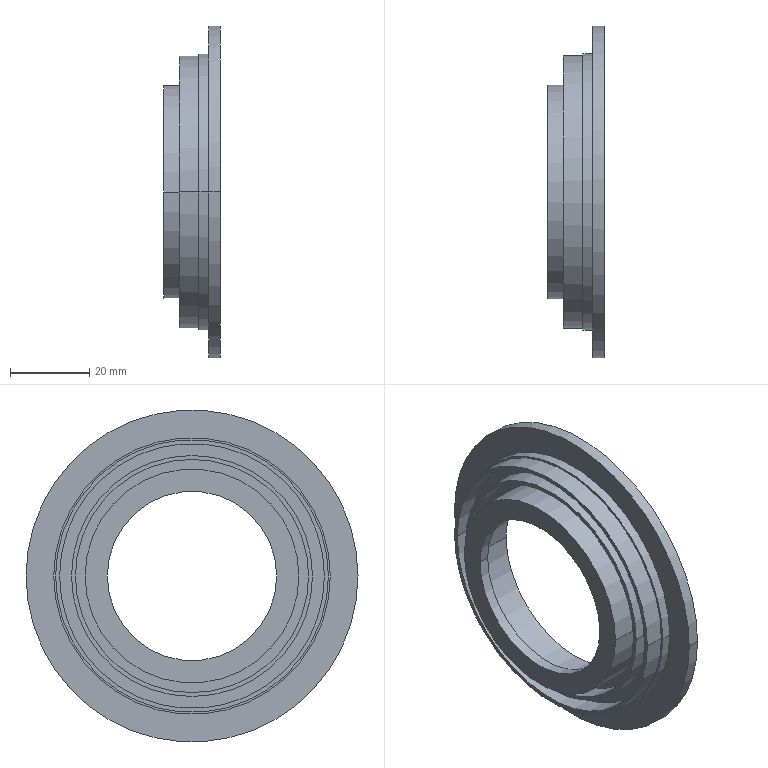Part | SolidWorks | features ICE 1, Revolution 1 | 1 solid | 30 faces | box 14.383 x 84 x 84 mm | volume 20141 mm3 | cylinder 20 | plane 10 | commonest cylinder face diameters 42.865 x2 49.1 x2 54.1 x2 59 x2 61 x2 62.852 x2
STEP:
#1=CARTESIAN_POINT('',(99.508,-34.5,0.));
#2=VERTEX_POINT('',#1);
#3=CARTESIAN_POINT('',(99.508,34.5,0.));
#4=VERTEX_POINT('',#3);
#5=CARTESIAN_POINT('',(99.508,0.,0.));
#6=DIRECTION('',(-1.,0.,0.));
#7=DIRECTION('',(0.,-1.,0.));
#8=AXIS2_PLACEMENT_3D('',#5,#6,#7);
#9=CIRCLE('',#8,34.5);
#10=EDGE_CURVE('',#2,#4,#9,.T.);
#11=ORIENTED_EDGE('',*,*,#10,.F.);
#12=CARTESIAN_POINT('',(104.508,-34.5,0.));
#13=VERTEX_POINT('',#12);
#14=CARTESIAN_POINT('',(99.508,-34.5,0.));
#15=DIRECTION('',(1.,0.,0.));
#16=VECTOR('',#15,1000.);
#17=LINE('',#14,#16);
#18=EDGE_CURVE('',#2,#13,#17,.T.);
#19=ORIENTED_EDGE('',*,*,#18,.T.);
#20=CARTESIAN_POINT('',(104.508,34.5,0.));
#21=VERTEX_POINT('',#20);
#22=CARTESIAN_POINT('',(104.508,0.,0.));
#23=DIRECTION('',(-1.,0.,0.));
#24=DIRECTION('',(0.,-1.,0.));
#25=AXIS2_PLACEMENT_3D('',#22,#23,#24);
#26=CIRCLE('',#25,34.5);
#27=EDGE_CURVE('',#13,#21,#26,.T.);
#28=ORIENTED_EDGE('',*,*,#27,.T.);
#29=CARTESIAN_POINT('',(99.508,34.5,0.));
#30=DIRECTION('',(1.,0.,0.));
#31=VECTOR('',#30,1000.);
#32=LINE('',#29,#31);
#33=EDGE_CURVE('',#4,#21,#32,.T.);
#34=ORIENTED_EDGE('',*,*,#33,.F.);
#35=EDGE_LOOP('',(#11,#19,#28,#34));
#36=FACE_OUTER_BOUND('',#35,.T.);
#37=CARTESIAN_POINT('',(99.508,0.,0.));
#38=DIRECTION('',(1.,0.,0.));
#39=DIRECTION('',(0.,1.,0.));
#40=AXIS2_PLACEMENT_3D('',#37,#38,#39);
#41=CYLINDRICAL_SURFACE('',#40,34.5);
#42=ADVANCED_FACE('',(#36),#41,.T.);
#43=CARTESIAN_POINT('',(99.508,33.5,0.));
#44=VERTEX_POINT('',#43);
#45=CARTESIAN_POINT('',(99.508,-33.5,0.));
#46=VERTEX_POINT('',#45);
#47=CARTESIAN_POINT('',(99.508,0.,0.));
#48=DIRECTION('',(-1.,0.,0.));
#49=DIRECTION('',(0.,-1.,0.));
#50=AXIS2_PLACEMENT_3D('',#47,#48,#49);
#51=CIRCLE('',#50,33.5);
#52=EDGE_CURVE('',#44,#46,#51,.T.);
#53=ORIENTED_EDGE('',*,*,#52,.T.);
#54=CARTESIAN_POINT('',(104.508,-33.5,0.));
#55=VERTEX_POINT('',#54);
#56=CARTESIAN_POINT('',(99.508,-33.5,0.));
#57=DIRECTION('',(1.,0.,0.));
#58=VECTOR('',#57,1000.);
#59=LINE('',#56,#58);
#60=EDGE_CURVE('',#46,#55,#59,.T.);
#61=ORIENTED_EDGE('',*,*,#60,.T.);
#62=CARTESIAN_POINT('',(104.508,33.5,0.));
#63=VERTEX_POINT('',#62);
#64=CARTESIAN_POINT('',(104.508,0.,0.));
#65=DIRECTION('',(1.,0.,0.));
#66=DIRECTION('',(0.,-1.,0.));
#67=AXIS2_PLACEMENT_3D('',#64,#65,#66);
#68=CIRCLE('',#67,33.5);
#69=EDGE_CURVE('',#55,#63,#68,.T.);
#70=ORIENTED_EDGE('',*,*,#69,.T.);
#71=CARTESIAN_POINT('',(99.508,33.5,0.));
#72=DIRECTION('',(1.,0.,0.));
#73=VECTOR('',#72,1000.);
#74=LINE('',#71,#73);
#75=EDGE_CURVE('',#44,#63,#74,.T.);
#76=ORIENTED_EDGE('',*,*,#75,.F.);
#77=EDGE_LOOP('',(#53,#61,#70,#76));
#78=FACE_OUTER_BOUND('',#77,.T.);
#79=CARTESIAN_POINT('',(99.508,0.,0.));
#80=DIRECTION('',(1.,0.,0.));
#81=DIRECTION('',(0.,1.,0.));
#82=AXIS2_PLACEMENT_3D('',#79,#80,#81);
#83=CYLINDRICAL_SURFACE('',#82,33.5);
#84=ADVANCED_FACE('',(#78),#83,.F.);
#85=CARTESIAN_POINT('',(99.508,-30.5,0.));
#86=VERTEX_POINT('',#85);
#87=CARTESIAN_POINT('',(99.508,30.5,0.));
#88=VERTEX_POINT('',#87);
#89=CARTESIAN_POINT('',(99.508,0.,0.));
#90=DIRECTION('',(-1.,0.,0.));
#91=DIRECTION('',(0.,-1.,0.));
#92=AXIS2_PLACEMENT_3D('',#89,#90,#91);
#93=CIRCLE('',#92,30.5);
#94=EDGE_CURVE('',#86,#88,#93,.T.);
#95=ORIENTED_EDGE('',*,*,#94,.F.);
#96=CARTESIAN_POINT('',(104.508,-30.5,0.));
#97=VERTEX_POINT('',#96);
#98=CARTESIAN_POINT('',(99.508,-30.5,0.));
#99=DIRECTION('',(1.,0.,0.));
#100=VECTOR('',#99,1000.);
#101=LINE('',#98,#100);
#102=EDGE_CURVE('',#86,#97,#101,.T.);
#103=ORIENTED_EDGE('',*,*,#102,.T.);
#104=CARTESIAN_POINT('',(104.508,30.5,0.));
#105=VERTEX_POINT('',#104);
#106=CARTESIAN_POINT('',(104.508,0.,0.));
#107=DIRECTION('',(-1.,0.,0.));
#108=DIRECTION('',(0.,-1.,0.));
#109=AXIS2_PLACEMENT_3D('',#106,#107,#108);
#110=CIRCLE('',#109,30.5);
#111=EDGE_CURVE('',#97,#105,#110,.T.);
#112=ORIENTED_EDGE('',*,*,#111,.T.);
#113=CARTESIAN_POINT('',(99.508,30.5,0.));
#114=DIRECTION('',(1.,0.,0.));
#115=VECTOR('',#114,1000.);
#116=LINE('',#113,#115);
#117=EDGE_CURVE('',#88,#105,#116,.T.);
#118=ORIENTED_EDGE('',*,*,#117,.F.);
#119=EDGE_LOOP('',(#95,#103,#112,#118));
#120=FACE_OUTER_BOUND('',#119,.T.);
#121=CARTESIAN_POINT('',(99.508,0.,0.));
#122=DIRECTION('',(1.,0.,0.));
#123=DIRECTION('',(0.,1.,0.));
#124=AXIS2_PLACEMENT_3D('',#121,#122,#123);
#125=CYLINDRICAL_SURFACE('',#124,30.5);
#126=ADVANCED_FACE('',(#120),#125,.T.);
#127=CARTESIAN_POINT('',(99.508,29.5,0.));
#128=VERTEX_POINT('',#127);
#129=CARTESIAN_POINT('',(99.508,-29.5,0.));
#130=VERTEX_POINT('',#129);
#131=CARTESIAN_POINT('',(99.508,0.,0.));
#132=DIRECTION('',(-1.,0.,0.));
#133=DIRECTION('',(0.,-1.,0.));
#134=AXIS2_PLACEMENT_3D('',#131,#132,#133);
#135=CIRCLE('',#134,29.5);
#136=EDGE_CURVE('',#128,#130,#135,.T.);
#137=ORIENTED_EDGE('',*,*,#136,.T.);
#138=CARTESIAN_POINT('',(104.508,-29.5,0.));
#139=VERTEX_POINT('',#138);
#140=CARTESIAN_POINT('',(99.508,-29.5,0.));
#141=DIRECTION('',(1.,0.,0.));
#142=VECTOR('',#141,1000.);
#143=LINE('',#140,#142);
#144=EDGE_CURVE('',#130,#139,#143,.T.);
#145=ORIENTED_EDGE('',*,*,#144,.T.);
#146=CARTESIAN_POINT('',(104.508,29.5,0.));
#147=VERTEX_POINT('',#146);
#148=CARTESIAN_POINT('',(104.508,0.,0.));
#149=DIRECTION('',(1.,0.,0.));
#150=DIRECTION('',(0.,-1.,0.));
#151=AXIS2_PLACEMENT_3D('',#148,#149,#150);
#152=CIRCLE('',#151,29.5);
#153=EDGE_CURVE('',#139,#147,#152,.T.);
#154=ORIENTED_EDGE('',*,*,#153,.T.);
#155=CARTESIAN_POINT('',(99.508,29.5,0.));
#156=DIRECTION('',(1.,0.,0.));
#157=VECTOR('',#156,1000.);
#158=LINE('',#155,#157);
#159=EDGE_CURVE('',#128,#147,#158,.T.);
#160=ORIENTED_EDGE('',*,*,#159,.F.);
#161=EDGE_LOOP('',(#137,#145,#154,#160));
#162=FACE_OUTER_BOUND('',#161,.T.);
#163=CARTESIAN_POINT('',(99.508,0.,0.));
#164=DIRECTION('',(1.,0.,0.));
#165=DIRECTION('',(0.,1.,0.));
#166=AXIS2_PLACEMENT_3D('',#163,#164,#165);
#167=CYLINDRICAL_SURFACE('',#166,29.5);
#168=ADVANCED_FACE('',(#162),#167,.F.);
#169=CARTESIAN_POINT('',(108.,-31.426,0.));
#170=VERTEX_POINT('',#169);
#171=CARTESIAN_POINT('',(108.,31.426,0.));
#172=VERTEX_POINT('',#171);
#173=CARTESIAN_POINT('',(108.,0.,0.));
#174=DIRECTION('',(1.,0.,0.));
#175=DIRECTION('',(0.,1.,0.));
#176=AXIS2_PLACEMENT_3D('',#173,#174,#175);
#177=CIRCLE('',#176,31.426);
#178=EDGE_CURVE('',#170,#172,#177,.T.);
#179=ORIENTED_EDGE('',*,*,#178,.F.);
#180=CARTESIAN_POINT('',(109.954,-31.426,0.));
#181=VERTEX_POINT('',#180);
#182=CARTESIAN_POINT('',(0.,-31.426,0.));
#183=DIRECTION('',(1.,0.,0.));
#184=VECTOR('',#183,1000.);
#185=LINE('',#182,#184);
#186=EDGE_CURVE('',#170,#181,#185,.T.);
#187=ORIENTED_EDGE('',*,*,#186,.T.);
#188=CARTESIAN_POINT('',(109.954,31.426,0.));
#189=VERTEX_POINT('',#188);
#190=CARTESIAN_POINT('',(109.954,0.,0.));
#191=DIRECTION('',(1.,0.,0.));
#192=DIRECTION('',(0.,1.,0.));
#193=AXIS2_PLACEMENT_3D('',#190,#191,#192);
#194=CIRCLE('',#193,31.426);
#195=EDGE_CURVE('',#181,#189,#194,.T.);
#196=ORIENTED_EDGE('',*,*,#195,.T.);
#197=CARTESIAN_POINT('',(0.,31.426,0.));
#198=DIRECTION('',(1.,0.,0.));
#199=VECTOR('',#198,1000.);
#200=LINE('',#197,#199);
#201=EDGE_CURVE('',#172,#189,#200,.T.);
#202=ORIENTED_EDGE('',*,*,#201,.F.);
#203=EDGE_LOOP('',(#179,#187,#196,#202));
#204=FACE_OUTER_BOUND('',#203,.T.);
#205=CARTESIAN_POINT('',(0.,0.,0.));
#206=DIRECTION('',(1.,0.,0.));
#207=DIRECTION('',(0.,1.,0.));
#208=AXIS2_PLACEMENT_3D('',#205,#206,#207);
#209=CYLINDRICAL_SURFACE('',#208,31.426);
#210=ADVANCED_FACE('',(#204),#209,.F.);
#211=CARTESIAN_POINT('',(98.286,-24.55,0.));
#212=VERTEX_POINT('',#211);
#213=CARTESIAN_POINT('',(98.286,24.55,0.));
#214=VERTEX_POINT('',#213);
#215=CARTESIAN_POINT('',(98.286,0.,0.));
#216=DIRECTION('',(1.,0.,0.));
#217=DIRECTION('',(0.,1.,0.));
#218=AXIS2_PLACEMENT_3D('',#215,#216,#217);
#219=CIRCLE('',#218,24.55);
#220=EDGE_CURVE('',#212,#214,#219,.T.);
#221=ORIENTED_EDGE('',*,*,#220,.F.);
#222=CARTESIAN_POINT('',(108.,-24.55,0.));
#223=VERTEX_POINT('',#222);
#224=CARTESIAN_POINT('',(0.,-24.55,0.));
#225=DIRECTION('',(1.,0.,0.));
#226=VECTOR('',#225,1000.);
#227=LINE('',#224,#226);
#228=EDGE_CURVE('',#212,#223,#227,.T.);
#229=ORIENTED_EDGE('',*,*,#228,.T.);
#230=CARTESIAN_POINT('',(108.,24.55,0.));
#231=VERTEX_POINT('',#230);
#232=CARTESIAN_POINT('',(108.,0.,0.));
#233=DIRECTION('',(1.,0.,0.));
#234=DIRECTION('',(0.,1.,0.));
#235=AXIS2_PLACEMENT_3D('',#232,#233,#234);
#236=CIRCLE('',#235,24.55);
#237=EDGE_CURVE('',#223,#231,#236,.T.);
#238=ORIENTED_EDGE('',*,*,#237,.T.);
#239=CARTESIAN_POINT('',(0.,24.55,0.));
#240=DIRECTION('',(1.,0.,0.));
#241=VECTOR('',#240,1000.);
#242=LINE('',#239,#241);
#243=EDGE_CURVE('',#214,#231,#242,.T.);
#244=ORIENTED_EDGE('',*,*,#243,.F.);
#245=EDGE_LOOP('',(#221,#229,#238,#244));
#246=FACE_OUTER_BOUND('',#245,.T.);
#247=CARTESIAN_POINT('',(0.,0.,0.));
#248=DIRECTION('',(1.,0.,0.));
#249=DIRECTION('',(0.,1.,0.));
#250=AXIS2_PLACEMENT_3D('',#247,#248,#249);
#251=CYLINDRICAL_SURFACE('',#250,24.55);
#252=ADVANCED_FACE('',(#246),#251,.F.);
#253=CARTESIAN_POINT('',(95.571,-21.433,0.));
#254=VERTEX_POINT('',#253);
#255=CARTESIAN_POINT('',(95.571,21.433,0.));
#256=VERTEX_POINT('',#255);
#257=CARTESIAN_POINT('',(95.571,0.,0.));
#258=DIRECTION('',(1.,0.,0.));
#259=DIRECTION('',(0.,1.,0.));
#260=AXIS2_PLACEMENT_3D('',#257,#258,#259);
#261=CIRCLE('',#260,21.433);
#262=EDGE_CURVE('',#254,#256,#261,.T.);
#263=ORIENTED_EDGE('',*,*,#262,.F.);
#264=CARTESIAN_POINT('',(98.286,-21.433,0.));
#265=VERTEX_POINT('',#264);
#266=CARTESIAN_POINT('',(0.,-21.433,0.));
#267=DIRECTION('',(1.,0.,0.));
#268=VECTOR('',#267,1000.);
#269=LINE('',#266,#268);
#270=EDGE_CURVE('',#254,#265,#269,.T.);
#271=ORIENTED_EDGE('',*,*,#270,.T.);
#272=CARTESIAN_POINT('',(98.286,21.433,0.));
#273=VERTEX_POINT('',#272);
#274=CARTESIAN_POINT('',(98.286,0.,0.));
#275=DIRECTION('',(1.,0.,0.));
#276=DIRECTION('',(0.,1.,0.));
#277=AXIS2_PLACEMENT_3D('',#274,#275,#276);
#278=CIRCLE('',#277,21.433);
#279=EDGE_CURVE('',#265,#273,#278,.T.);
#280=ORIENTED_EDGE('',*,*,#279,.T.);
#281=CARTESIAN_POINT('',(0.,21.433,0.));
#282=DIRECTION('',(1.,0.,0.));
#283=VECTOR('',#282,1000.);
#284=LINE('',#281,#283);
#285=EDGE_CURVE('',#256,#273,#284,.T.);
#286=ORIENTED_EDGE('',*,*,#285,.F.);
#287=EDGE_LOOP('',(#263,#271,#280,#286));
#288=FACE_OUTER_BOUND('',#287,.T.);
#289=CARTESIAN_POINT('',(0.,0.,0.));
#290=DIRECTION('',(1.,0.,0.));
#291=DIRECTION('',(0.,1.,0.));
#292=AXIS2_PLACEMENT_3D('',#289,#290,#291);
#293=CYLINDRICAL_SURFACE('',#292,21.433);
#294=ADVANCED_FACE('',(#288),#293,.F.);
#295=CARTESIAN_POINT('',(95.571,27.05,0.));
#296=VERTEX_POINT('',#295);
#297=CARTESIAN_POINT('',(95.571,-27.05,0.));
#298=VERTEX_POINT('',#297);
#299=CARTESIAN_POINT('',(95.571,0.,0.));
#300=DIRECTION('',(1.,0.,0.));
#301=DIRECTION('',(0.,1.,0.));
#302=AXIS2_PLACEMENT_3D('',#299,#300,#301);
#303=CIRCLE('',#302,27.05);
#304=EDGE_CURVE('',#296,#298,#303,.T.);
#305=ORIENTED_EDGE('',*,*,#304,.T.);
#306=CARTESIAN_POINT('',(104.508,-27.05,0.));
#307=VERTEX_POINT('',#306);
#308=CARTESIAN_POINT('',(0.,-27.05,0.));
#309=DIRECTION('',(1.,0.,0.));
#310=VECTOR('',#309,1000.);
#311=LINE('',#308,#310);
#312=EDGE_CURVE('',#298,#307,#311,.T.);
#313=ORIENTED_EDGE('',*,*,#312,.T.);
#314=CARTESIAN_POINT('',(104.508,27.05,0.));
#315=VERTEX_POINT('',#314);
#316=CARTESIAN_POINT('',(104.508,0.,0.));
#317=DIRECTION('',(1.,0.,0.));
#318=DIRECTION('',(0.,1.,0.));
#319=AXIS2_PLACEMENT_3D('',#316,#317,#318);
#320=CIRCLE('',#319,27.05);
#321=EDGE_CURVE('',#315,#307,#320,.T.);
#322=ORIENTED_EDGE('',*,*,#321,.F.);
#323=CARTESIAN_POINT('',(0.,27.05,0.));
#324=DIRECTION('',(1.,0.,0.));
#325=VECTOR('',#324,1000.);
#326=LINE('',#323,#325);
#327=EDGE_CURVE('',#296,#315,#326,.T.);
#328=ORIENTED_EDGE('',*,*,#327,.F.);
#329=EDGE_LOOP('',(#305,#313,#322,#328));
#330=FACE_OUTER_BOUND('',#329,.T.);
#331=CARTESIAN_POINT('',(0.,0.,0.));
#332=DIRECTION('',(1.,0.,0.));
#333=DIRECTION('',(0.,1.,0.));
#334=AXIS2_PLACEMENT_3D('',#331,#332,#333);
#335=CYLINDRICAL_SURFACE('',#334,27.05);
#336=ADVANCED_FACE('',(#330),#335,.T.);
#337=CARTESIAN_POINT('',(104.508,35.,0.));
#338=VERTEX_POINT('',#337);
#339=CARTESIAN_POINT('',(104.508,-35.,0.));
#340=VERTEX_POINT('',#339);
#341=CARTESIAN_POINT('',(104.508,0.,0.));
#342=DIRECTION('',(1.,0.,0.));
#343=DIRECTION('',(0.,1.,0.));
#344=AXIS2_PLACEMENT_3D('',#341,#342,#343);
#345=CIRCLE('',#344,35.);
#346=EDGE_CURVE('',#338,#340,#345,.T.);
#347=ORIENTED_EDGE('',*,*,#346,.T.);
#348=CARTESIAN_POINT('',(107.,-35.,0.));
#349=VERTEX_POINT('',#348);
#350=CARTESIAN_POINT('',(0.,-35.,0.));
#351=DIRECTION('',(1.,0.,0.));
#352=VECTOR('',#351,1000.);
#353=LINE('',#350,#352);
#354=EDGE_CURVE('',#340,#349,#353,.T.);
#355=ORIENTED_EDGE('',*,*,#354,.T.);
#356=CARTESIAN_POINT('',(107.,35.,0.));
#357=VERTEX_POINT('',#356);
#358=CARTESIAN_POINT('',(107.,0.,0.));
#359=DIRECTION('',(1.,0.,0.));
#360=DIRECTION('',(0.,1.,0.));
#361=AXIS2_PLACEMENT_3D('',#358,#359,#360);
#362=CIRCLE('',#361,35.);
#363=EDGE_CURVE('',#357,#349,#362,.T.);
#364=ORIENTED_EDGE('',*,*,#363,.F.);
#365=CARTESIAN_POINT('',(0.,35.,0.));
#366=DIRECTION('',(1.,0.,0.));
#367=VECTOR('',#366,1000.);
#368=LINE('',#365,#367);
#369=EDGE_CURVE('',#338,#357,#368,.T.);
#370=ORIENTED_EDGE('',*,*,#369,.F.);
#371=EDGE_LOOP('',(#347,#355,#364,#370));
#372=FACE_OUTER_BOUND('',#371,.T.);
#373=CARTESIAN_POINT('',(0.,0.,0.));
#374=DIRECTION('',(1.,0.,0.));
#375=DIRECTION('',(0.,1.,0.));
#376=AXIS2_PLACEMENT_3D('',#373,#374,#375);
#377=CYLINDRICAL_SURFACE('',#376,35.);
#378=ADVANCED_FACE('',(#372),#377,.T.);
#379=CARTESIAN_POINT('',(107.,42.,0.));
#380=VERTEX_POINT('',#379);
#381=CARTESIAN_POINT('',(107.,-42.,0.));
#382=VERTEX_POINT('',#381);
#383=CARTESIAN_POINT('',(107.,0.,0.));
#384=DIRECTION('',(1.,0.,0.));
#385=DIRECTION('',(0.,1.,0.));
#386=AXIS2_PLACEMENT_3D('',#383,#384,#385);
#387=CIRCLE('',#386,42.);
#388=EDGE_CURVE('',#380,#382,#387,.T.);
#389=ORIENTED_EDGE('',*,*,#388,.T.);
#390=CARTESIAN_POINT('',(109.954,-42.,0.));
#391=VERTEX_POINT('',#390);
#392=CARTESIAN_POINT('',(0.,-42.,0.));
#393=DIRECTION('',(1.,0.,0.));
#394=VECTOR('',#393,1000.);
#395=LINE('',#392,#394);
#396=EDGE_CURVE('',#382,#391,#395,.T.);
#397=ORIENTED_EDGE('',*,*,#396,.T.);
#398=CARTESIAN_POINT('',(109.954,42.,0.));
#399=VERTEX_POINT('',#398);
#400=CARTESIAN_POINT('',(109.954,0.,0.));
#401=DIRECTION('',(1.,0.,0.));
#402=DIRECTION('',(0.,1.,0.));
#403=AXIS2_PLACEMENT_3D('',#400,#401,#402);
#404=CIRCLE('',#403,42.);
#405=EDGE_CURVE('',#399,#391,#404,.T.);
#406=ORIENTED_EDGE('',*,*,#405,.F.);
#407=CARTESIAN_POINT('',(0.,42.,0.));
#408=DIRECTION('',(1.,0.,0.));
#409=VECTOR('',#408,1000.);
#410=LINE('',#407,#409);
#411=EDGE_CURVE('',#380,#399,#410,.T.);
#412=ORIENTED_EDGE('',*,*,#411,.F.);
#413=EDGE_LOOP('',(#389,#397,#406,#412));
#414=FACE_OUTER_BOUND('',#413,.T.);
#415=CARTESIAN_POINT('',(0.,0.,0.));
#416=DIRECTION('',(1.,0.,0.));
#417=DIRECTION('',(0.,1.,0.));
#418=AXIS2_PLACEMENT_3D('',#415,#416,#417);
#419=CYLINDRICAL_SURFACE('',#418,42.);
#420=ADVANCED_FACE('',(#414),#419,.T.);
#421=CARTESIAN_POINT('',(104.508,0.,0.));
#422=DIRECTION('',(-1.,0.,0.));
#423=DIRECTION('',(0.,-1.,0.));
#424=AXIS2_PLACEMENT_3D('',#421,#422,#423);
#425=CIRCLE('',#424,30.5);
#426=EDGE_CURVE('',#105,#97,#425,.T.);
#427=ORIENTED_EDGE('',*,*,#426,.F.);
#428=ORIENTED_EDGE('',*,*,#111,.F.);
#429=EDGE_LOOP('',(#427,#428));
#430=FACE_BOUND('',#429,.T.);
#431=CARTESIAN_POINT('',(104.508,0.,0.));
#432=DIRECTION('',(1.,0.,0.));
#433=DIRECTION('',(0.,-1.,0.));
#434=AXIS2_PLACEMENT_3D('',#431,#432,#433);
#435=CIRCLE('',#434,33.5);
#436=EDGE_CURVE('',#63,#55,#435,.T.);
#437=ORIENTED_EDGE('',*,*,#436,.F.);
#438=ORIENTED_EDGE('',*,*,#69,.F.);
#439=EDGE_LOOP('',(#437,#438));
#440=FACE_OUTER_BOUND('',#439,.T.);
#441=CARTESIAN_POINT('',(104.508,35.,0.));
#442=DIRECTION('',(-1.,0.,0.));
#443=DIRECTION('',(0.,-1.,0.));
#444=AXIS2_PLACEMENT_3D('',#441,#442,#443);
#445=PLANE('',#444);
#446=ADVANCED_FACE('',(#430,#440),#445,.T.);
#447=ORIENTED_EDGE('',*,*,#321,.T.);
#448=CARTESIAN_POINT('',(104.508,0.,0.));
#449=DIRECTION('',(1.,0.,0.));
#450=DIRECTION('',(0.,1.,0.));
#451=AXIS2_PLACEMENT_3D('',#448,#449,#450);
#452=CIRCLE('',#451,27.05);
#453=EDGE_CURVE('',#307,#315,#452,.T.);
#454=ORIENTED_EDGE('',*,*,#453,.T.);
#455=EDGE_LOOP('',(#447,#454));
#456=FACE_BOUND('',#455,.T.);
#457=CARTESIAN_POINT('',(104.508,0.,0.));
#458=DIRECTION('',(1.,0.,0.));
#459=DIRECTION('',(0.,-1.,0.));
#460=AXIS2_PLACEMENT_3D('',#457,#458,#459);
#461=CIRCLE('',#460,29.5);
#462=EDGE_CURVE('',#147,#139,#461,.T.);
#463=ORIENTED_EDGE('',*,*,#462,.F.);
#464=ORIENTED_EDGE('',*,*,#153,.F.);
#465=EDGE_LOOP('',(#463,#464));
#466=FACE_OUTER_BOUND('',#465,.T.);
#467=CARTESIAN_POINT('',(104.508,35.,0.));
#468=DIRECTION('',(-1.,0.,0.));
#469=DIRECTION('',(0.,-1.,0.));
#470=AXIS2_PLACEMENT_3D('',#467,#468,#469);
#471=PLANE('',#470);
#472=ADVANCED_FACE('',(#456,#466),#471,.T.);
#473=ORIENTED_EDGE('',*,*,#396,.F.);
#474=CARTESIAN_POINT('',(107.,0.,0.));
#475=DIRECTION('',(1.,0.,0.));
#476=DIRECTION('',(0.,1.,0.));
#477=AXIS2_PLACEMENT_3D('',#474,#475,#476);
#478=CIRCLE('',#477,42.);
#479=EDGE_CURVE('',#382,#380,#478,.T.);
#480=ORIENTED_EDGE('',*,*,#479,.T.);
#481=ORIENTED_EDGE('',*,*,#411,.T.);
#482=CARTESIAN_POINT('',(109.954,0.,0.));
#483=DIRECTION('',(1.,0.,0.));
#484=DIRECTION('',(0.,1.,0.));
#485=AXIS2_PLACEMENT_3D('',#482,#483,#484);
#486=CIRCLE('',#485,42.);
#487=EDGE_CURVE('',#391,#399,#486,.T.);
#488=ORIENTED_EDGE('',*,*,#487,.F.);
#489=EDGE_LOOP('',(#473,#480,#481,#488));
#490=FACE_OUTER_BOUND('',#489,.T.);
#491=CARTESIAN_POINT('',(0.,0.,0.));
#492=DIRECTION('',(1.,0.,0.));
#493=DIRECTION('',(0.,1.,0.));
#494=AXIS2_PLACEMENT_3D('',#491,#492,#493);
#495=CYLINDRICAL_SURFACE('',#494,42.);
#496=ADVANCED_FACE('',(#490),#495,.T.);
#497=ORIENTED_EDGE('',*,*,#363,.T.);
#498=CARTESIAN_POINT('',(107.,0.,0.));
#499=DIRECTION('',(1.,0.,0.));
#500=DIRECTION('',(0.,1.,0.));
#501=AXIS2_PLACEMENT_3D('',#498,#499,#500);
#502=CIRCLE('',#501,35.);
#503=EDGE_CURVE('',#349,#357,#502,.T.);
#504=ORIENTED_EDGE('',*,*,#503,.T.);
#505=EDGE_LOOP('',(#497,#504));
#506=FACE_BOUND('',#505,.T.);
#507=ORIENTED_EDGE('',*,*,#388,.F.);
#508=ORIENTED_EDGE('',*,*,#479,.F.);
#509=EDGE_LOOP('',(#507,#508));
#510=FACE_OUTER_BOUND('',#509,.T.);
#511=CARTESIAN_POINT('',(107.,42.,0.));
#512=DIRECTION('',(-1.,0.,0.));
#513=DIRECTION('',(0.,-1.,0.));
#514=AXIS2_PLACEMENT_3D('',#511,#512,#513);
#515=PLANE('',#514);
#516=ADVANCED_FACE('',(#506,#510),#515,.T.);
#517=ORIENTED_EDGE('',*,*,#354,.F.);
#518=CARTESIAN_POINT('',(104.508,0.,0.));
#519=DIRECTION('',(1.,0.,0.));
#520=DIRECTION('',(0.,1.,0.));
#521=AXIS2_PLACEMENT_3D('',#518,#519,#520);
#522=CIRCLE('',#521,35.);
#523=EDGE_CURVE('',#340,#338,#522,.T.);
#524=ORIENTED_EDGE('',*,*,#523,.T.);
#525=ORIENTED_EDGE('',*,*,#369,.T.);
#526=ORIENTED_EDGE('',*,*,#503,.F.);
#527=EDGE_LOOP('',(#517,#524,#525,#526));
#528=FACE_OUTER_BOUND('',#527,.T.);
#529=CARTESIAN_POINT('',(0.,0.,0.));
#530=DIRECTION('',(1.,0.,0.));
#531=DIRECTION('',(0.,1.,0.));
#532=AXIS2_PLACEMENT_3D('',#529,#530,#531);
#533=CYLINDRICAL_SURFACE('',#532,35.);
#534=ADVANCED_FACE('',(#528),#533,.T.);
#535=CARTESIAN_POINT('',(104.508,0.,0.));
#536=DIRECTION('',(-1.,0.,0.));
#537=DIRECTION('',(0.,-1.,0.));
#538=AXIS2_PLACEMENT_3D('',#535,#536,#537);
#539=CIRCLE('',#538,34.5);
#540=EDGE_CURVE('',#21,#13,#539,.T.);
#541=ORIENTED_EDGE('',*,*,#540,.F.);
#542=ORIENTED_EDGE('',*,*,#27,.F.);
#543=EDGE_LOOP('',(#541,#542));
#544=FACE_BOUND('',#543,.T.);
#545=ORIENTED_EDGE('',*,*,#346,.F.);
#546=ORIENTED_EDGE('',*,*,#523,.F.);
#547=EDGE_LOOP('',(#545,#546));
#548=FACE_OUTER_BOUND('',#547,.T.);
#549=CARTESIAN_POINT('',(104.508,35.,0.));
#550=DIRECTION('',(-1.,0.,0.));
#551=DIRECTION('',(0.,-1.,0.));
#552=AXIS2_PLACEMENT_3D('',#549,#550,#551);
#553=PLANE('',#552);
#554=ADVANCED_FACE('',(#544,#548),#553,.T.);
#555=ORIENTED_EDGE('',*,*,#312,.F.);
#556=CARTESIAN_POINT('',(95.571,0.,0.));
#557=DIRECTION('',(1.,0.,0.));
#558=DIRECTION('',(0.,1.,0.));
#559=AXIS2_PLACEMENT_3D('',#556,#557,#558);
#560=CIRCLE('',#559,27.05);
#561=EDGE_CURVE('',#298,#296,#560,.T.);
#562=ORIENTED_EDGE('',*,*,#561,.T.);
#563=ORIENTED_EDGE('',*,*,#327,.T.);
#564=ORIENTED_EDGE('',*,*,#453,.F.);
#565=EDGE_LOOP('',(#555,#562,#563,#564));
#566=FACE_OUTER_BOUND('',#565,.T.);
#567=CARTESIAN_POINT('',(0.,0.,0.));
#568=DIRECTION('',(1.,0.,0.));
#569=DIRECTION('',(0.,1.,0.));
#570=AXIS2_PLACEMENT_3D('',#567,#568,#569);
#571=CYLINDRICAL_SURFACE('',#570,27.05);
#572=ADVANCED_FACE('',(#566),#571,.T.);
#573=CARTESIAN_POINT('',(95.571,0.,0.));
#574=DIRECTION('',(1.,0.,0.));
#575=DIRECTION('',(0.,1.,0.));
#576=AXIS2_PLACEMENT_3D('',#573,#574,#575);
#577=CIRCLE('',#576,21.433);
#578=EDGE_CURVE('',#256,#254,#577,.T.);
#579=ORIENTED_EDGE('',*,*,#578,.T.);
#580=ORIENTED_EDGE('',*,*,#262,.T.);
#581=EDGE_LOOP('',(#579,#580));
#582=FACE_BOUND('',#581,.T.);
#583=ORIENTED_EDGE('',*,*,#304,.F.);
#584=ORIENTED_EDGE('',*,*,#561,.F.);
#585=EDGE_LOOP('',(#583,#584));
#586=FACE_OUTER_BOUND('',#585,.T.);
#587=CARTESIAN_POINT('',(95.571,27.05,0.));
#588=DIRECTION('',(-1.,0.,0.));
#589=DIRECTION('',(0.,-1.,0.));
#590=AXIS2_PLACEMENT_3D('',#587,#588,#589);
#591=PLANE('',#590);
#592=ADVANCED_FACE('',(#582,#586),#591,.T.);
#593=ORIENTED_EDGE('',*,*,#270,.F.);
#594=ORIENTED_EDGE('',*,*,#578,.F.);
#595=ORIENTED_EDGE('',*,*,#285,.T.);
#596=CARTESIAN_POINT('',(98.286,0.,0.));
#597=DIRECTION('',(1.,0.,0.));
#598=DIRECTION('',(0.,1.,0.));
#599=AXIS2_PLACEMENT_3D('',#596,#597,#598);
#600=CIRCLE('',#599,21.433);
#601=EDGE_CURVE('',#273,#265,#600,.T.);
#602=ORIENTED_EDGE('',*,*,#601,.T.);
#603=EDGE_LOOP('',(#593,#594,#595,#602));
#604=FACE_OUTER_BOUND('',#603,.T.);
#605=CARTESIAN_POINT('',(0.,0.,0.));
#606=DIRECTION('',(1.,0.,0.));
#607=DIRECTION('',(0.,1.,0.));
#608=AXIS2_PLACEMENT_3D('',#605,#606,#607);
#609=CYLINDRICAL_SURFACE('',#608,21.433);
#610=ADVANCED_FACE('',(#604),#609,.F.);
#611=CARTESIAN_POINT('',(98.286,0.,0.));
#612=DIRECTION('',(1.,0.,0.));
#613=DIRECTION('',(0.,1.,0.));
#614=AXIS2_PLACEMENT_3D('',#611,#612,#613);
#615=CIRCLE('',#614,24.55);
#616=EDGE_CURVE('',#214,#212,#615,.T.);
#617=ORIENTED_EDGE('',*,*,#616,.T.);
#618=ORIENTED_EDGE('',*,*,#220,.T.);
#619=EDGE_LOOP('',(#617,#618));
#620=FACE_OUTER_BOUND('',#619,.T.);
#621=ORIENTED_EDGE('',*,*,#601,.F.);
#622=ORIENTED_EDGE('',*,*,#279,.F.);
#623=EDGE_LOOP('',(#621,#622));
#624=FACE_BOUND('',#623,.T.);
#625=CARTESIAN_POINT('',(98.286,21.433,0.));
#626=DIRECTION('',(1.,0.,0.));
#627=DIRECTION('',(0.,1.,0.));
#628=AXIS2_PLACEMENT_3D('',#625,#626,#627);
#629=PLANE('',#628);
#630=ADVANCED_FACE('',(#620,#624),#629,.T.);
#631=ORIENTED_EDGE('',*,*,#228,.F.);
#632=ORIENTED_EDGE('',*,*,#616,.F.);
#633=ORIENTED_EDGE('',*,*,#243,.T.);
#634=CARTESIAN_POINT('',(108.,0.,0.));
#635=DIRECTION('',(1.,0.,0.));
#636=DIRECTION('',(0.,1.,0.));
#637=AXIS2_PLACEMENT_3D('',#634,#635,#636);
#638=CIRCLE('',#637,24.55);
#639=EDGE_CURVE('',#231,#223,#638,.T.);
#640=ORIENTED_EDGE('',*,*,#639,.T.);
#641=EDGE_LOOP('',(#631,#632,#633,#640));
#642=FACE_OUTER_BOUND('',#641,.T.);
#643=CARTESIAN_POINT('',(0.,0.,0.));
#644=DIRECTION('',(1.,0.,0.));
#645=DIRECTION('',(0.,1.,0.));
#646=AXIS2_PLACEMENT_3D('',#643,#644,#645);
#647=CYLINDRICAL_SURFACE('',#646,24.55);
#648=ADVANCED_FACE('',(#642),#647,.F.);
#649=CARTESIAN_POINT('',(108.,0.,0.));
#650=DIRECTION('',(1.,0.,0.));
#651=DIRECTION('',(0.,1.,0.));
#652=AXIS2_PLACEMENT_3D('',#649,#650,#651);
#653=CIRCLE('',#652,31.426);
#654=EDGE_CURVE('',#172,#170,#653,.T.);
#655=ORIENTED_EDGE('',*,*,#654,.T.);
#656=ORIENTED_EDGE('',*,*,#178,.T.);
#657=EDGE_LOOP('',(#655,#656));
#658=FACE_OUTER_BOUND('',#657,.T.);
#659=ORIENTED_EDGE('',*,*,#639,.F.);
#660=ORIENTED_EDGE('',*,*,#237,.F.);
#661=EDGE_LOOP('',(#659,#660));
#662=FACE_BOUND('',#661,.T.);
#663=CARTESIAN_POINT('',(108.,31.426,0.));
#664=DIRECTION('',(1.,0.,0.));
#665=DIRECTION('',(0.,1.,0.));
#666=AXIS2_PLACEMENT_3D('',#663,#664,#665);
#667=PLANE('',#666);
#668=ADVANCED_FACE('',(#658,#662),#667,.T.);
#669=ORIENTED_EDGE('',*,*,#186,.F.);
#670=ORIENTED_EDGE('',*,*,#654,.F.);
#671=ORIENTED_EDGE('',*,*,#201,.T.);
#672=CARTESIAN_POINT('',(109.954,0.,0.));
#673=DIRECTION('',(1.,0.,0.));
#674=DIRECTION('',(0.,1.,0.));
#675=AXIS2_PLACEMENT_3D('',#672,#673,#674);
#676=CIRCLE('',#675,31.426);
#677=EDGE_CURVE('',#189,#181,#676,.T.);
#678=ORIENTED_EDGE('',*,*,#677,.T.);
#679=EDGE_LOOP('',(#669,#670,#671,#678));
#680=FACE_OUTER_BOUND('',#679,.T.);
#681=CARTESIAN_POINT('',(0.,0.,0.));
#682=DIRECTION('',(1.,0.,0.));
#683=DIRECTION('',(0.,1.,0.));
#684=AXIS2_PLACEMENT_3D('',#681,#682,#683);
#685=CYLINDRICAL_SURFACE('',#684,31.426);
#686=ADVANCED_FACE('',(#680),#685,.F.);
#687=ORIENTED_EDGE('',*,*,#405,.T.);
#688=ORIENTED_EDGE('',*,*,#487,.T.);
#689=EDGE_LOOP('',(#687,#688));
#690=FACE_OUTER_BOUND('',#689,.T.);
#691=ORIENTED_EDGE('',*,*,#677,.F.);
#692=ORIENTED_EDGE('',*,*,#195,.F.);
#693=EDGE_LOOP('',(#691,#692));
#694=FACE_BOUND('',#693,.T.);
#695=CARTESIAN_POINT('',(109.954,31.426,0.));
#696=DIRECTION('',(1.,0.,0.));
#697=DIRECTION('',(0.,1.,0.));
#698=AXIS2_PLACEMENT_3D('',#695,#696,#697);
#699=PLANE('',#698);
#700=ADVANCED_FACE('',(#690,#694),#699,.T.);
#701=ORIENTED_EDGE('',*,*,#144,.F.);
#702=CARTESIAN_POINT('',(99.508,0.,0.));
#703=DIRECTION('',(-1.,0.,0.));
#704=DIRECTION('',(0.,-1.,0.));
#705=AXIS2_PLACEMENT_3D('',#702,#703,#704);
#706=CIRCLE('',#705,29.5);
#707=EDGE_CURVE('',#130,#128,#706,.T.);
#708=ORIENTED_EDGE('',*,*,#707,.T.);
#709=ORIENTED_EDGE('',*,*,#159,.T.);
#710=ORIENTED_EDGE('',*,*,#462,.T.);
#711=EDGE_LOOP('',(#701,#708,#709,#710));
#712=FACE_OUTER_BOUND('',#711,.T.);
#713=CARTESIAN_POINT('',(99.508,0.,0.));
#714=DIRECTION('',(1.,0.,0.));
#715=DIRECTION('',(0.,1.,0.));
#716=AXIS2_PLACEMENT_3D('',#713,#714,#715);
#717=CYLINDRICAL_SURFACE('',#716,29.5);
#718=ADVANCED_FACE('',(#712),#717,.F.);
#719=ORIENTED_EDGE('',*,*,#102,.F.);
#720=CARTESIAN_POINT('',(99.508,0.,0.));
#721=DIRECTION('',(-1.,0.,0.));
#722=DIRECTION('',(0.,-1.,0.));
#723=AXIS2_PLACEMENT_3D('',#720,#721,#722);
#724=CIRCLE('',#723,30.5);
#725=EDGE_CURVE('',#88,#86,#724,.T.);
#726=ORIENTED_EDGE('',*,*,#725,.F.);
#727=ORIENTED_EDGE('',*,*,#117,.T.);
#728=ORIENTED_EDGE('',*,*,#426,.T.);
#729=EDGE_LOOP('',(#719,#726,#727,#728));
#730=FACE_OUTER_BOUND('',#729,.T.);
#731=CARTESIAN_POINT('',(99.508,0.,0.));
#732=DIRECTION('',(1.,0.,0.));
#733=DIRECTION('',(0.,1.,0.));
#734=AXIS2_PLACEMENT_3D('',#731,#732,#733);
#735=CYLINDRICAL_SURFACE('',#734,30.5);
#736=ADVANCED_FACE('',(#730),#735,.T.);
#737=ORIENTED_EDGE('',*,*,#136,.F.);
#738=ORIENTED_EDGE('',*,*,#707,.F.);
#739=EDGE_LOOP('',(#737,#738));
#740=FACE_BOUND('',#739,.T.);
#741=ORIENTED_EDGE('',*,*,#725,.T.);
#742=ORIENTED_EDGE('',*,*,#94,.T.);
#743=EDGE_LOOP('',(#741,#742));
#744=FACE_OUTER_BOUND('',#743,.T.);
#745=CARTESIAN_POINT('',(99.508,0.,0.));
#746=DIRECTION('',(-1.,0.,0.));
#747=DIRECTION('',(0.,-1.,0.));
#748=AXIS2_PLACEMENT_3D('',#745,#746,#747);
#749=PLANE('',#748);
#750=ADVANCED_FACE('',(#740,#744),#749,.T.);
#751=ORIENTED_EDGE('',*,*,#60,.F.);
#752=CARTESIAN_POINT('',(99.508,0.,0.));
#753=DIRECTION('',(-1.,0.,0.));
#754=DIRECTION('',(0.,-1.,0.));
#755=AXIS2_PLACEMENT_3D('',#752,#753,#754);
#756=CIRCLE('',#755,33.5);
#757=EDGE_CURVE('',#46,#44,#756,.T.);
#758=ORIENTED_EDGE('',*,*,#757,.T.);
#759=ORIENTED_EDGE('',*,*,#75,.T.);
#760=ORIENTED_EDGE('',*,*,#436,.T.);
#761=EDGE_LOOP('',(#751,#758,#759,#760));
#762=FACE_OUTER_BOUND('',#761,.T.);
#763=CARTESIAN_POINT('',(99.508,0.,0.));
#764=DIRECTION('',(1.,0.,0.));
#765=DIRECTION('',(0.,1.,0.));
#766=AXIS2_PLACEMENT_3D('',#763,#764,#765);
#767=CYLINDRICAL_SURFACE('',#766,33.5);
#768=ADVANCED_FACE('',(#762),#767,.F.);
#769=ORIENTED_EDGE('',*,*,#18,.F.);
#770=CARTESIAN_POINT('',(99.508,0.,0.));
#771=DIRECTION('',(-1.,0.,0.));
#772=DIRECTION('',(0.,-1.,0.));
#773=AXIS2_PLACEMENT_3D('',#770,#771,#772);
#774=CIRCLE('',#773,34.5);
#775=EDGE_CURVE('',#4,#2,#774,.T.);
#776=ORIENTED_EDGE('',*,*,#775,.F.);
#777=ORIENTED_EDGE('',*,*,#33,.T.);
#778=ORIENTED_EDGE('',*,*,#540,.T.);
#779=EDGE_LOOP('',(#769,#776,#777,#778));
#780=FACE_OUTER_BOUND('',#779,.T.);
#781=CARTESIAN_POINT('',(99.508,0.,0.));
#782=DIRECTION('',(1.,0.,0.));
#783=DIRECTION('',(0.,1.,0.));
#784=AXIS2_PLACEMENT_3D('',#781,#782,#783);
#785=CYLINDRICAL_SURFACE('',#784,34.5);
#786=ADVANCED_FACE('',(#780),#785,.T.);
#787=ORIENTED_EDGE('',*,*,#52,.F.);
#788=ORIENTED_EDGE('',*,*,#757,.F.);
#789=EDGE_LOOP('',(#787,#788));
#790=FACE_BOUND('',#789,.T.);
#791=ORIENTED_EDGE('',*,*,#775,.T.);
#792=ORIENTED_EDGE('',*,*,#10,.T.);
#793=EDGE_LOOP('',(#791,#792));
#794=FACE_OUTER_BOUND('',#793,.T.);
#795=CARTESIAN_POINT('',(99.508,0.,0.));
#796=DIRECTION('',(-1.,0.,0.));
#797=DIRECTION('',(0.,-1.,0.));
#798=AXIS2_PLACEMENT_3D('',#795,#796,#797);
#799=PLANE('',#798);
#800=ADVANCED_FACE('',(#790,#794),#799,.T.);
#801=CLOSED_SHELL('',(#42,#84,#126,#168,#210,#252,#294,#336,#378,#420,#446,#472,#496,#516,#534,#554,#572,#592,#610,#630,#648,#668,#686,#700,#718,#736,#750,#768,#786,#800));
#802=MANIFOLD_SOLID_BREP('',#801);
#803=CARTESIAN_POINT('',(0.,0.,0.));
#804=DIRECTION('',(0.,0.,1.));
#805=DIRECTION('',(1.,0.,0.));
#806=AXIS2_PLACEMENT_3D('',#803,#804,#805);
#807=(LENGTH_UNIT()NAMED_UNIT(*)SI_UNIT(.MILLI.,.METRE.));
#808=UNCERTAINTY_MEASURE_WITH_UNIT(LENGTH_MEASURE(0.00001),#807,'','');
#809=(NAMED_UNIT(*)PLANE_ANGLE_UNIT()SI_UNIT($,.RADIAN.));
#810=(NAMED_UNIT(*)SI_UNIT($,.STERADIAN.)SOLID_ANGLE_UNIT());
#811=(GEOMETRIC_REPRESENTATION_CONTEXT(3)GLOBAL_UNCERTAINTY_ASSIGNED_CONTEXT((#808))GLOBAL_UNIT_ASSIGNED_CONTEXT((#807,#809,#810))REPRESENTATION_CONTEXT('',''));
#812=ADVANCED_BREP_SHAPE_REPRESENTATION('',(#802,#806),#811);